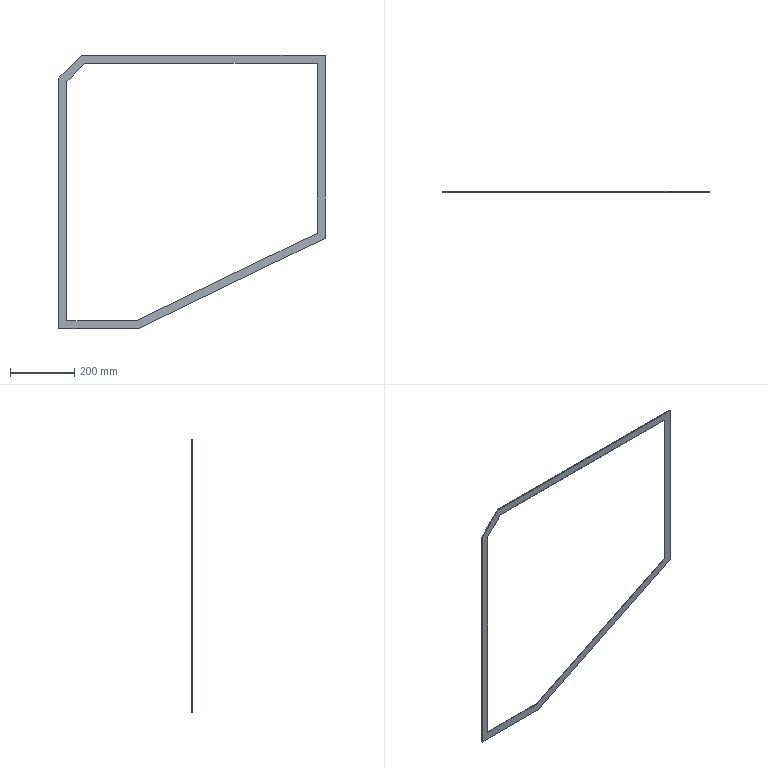Part | NX | features BREP 1 | 1 solid | 14 faces | box 830.914 x 2 x 852.689 mm | volume 150814 mm3 | plane 14
STEP:
#1=CARTESIAN_POINT('',(802.673,-691.5,466.003));
#2=VERTEX_POINT('',#1);
#3=CARTESIAN_POINT('',(802.673,-691.5,1212.752));
#4=VERTEX_POINT('',#3);
#5=CARTESIAN_POINT('',(802.673,-691.5,839.378));
#6=DIRECTION('',(0.,0.,1.));
#7=VECTOR('',#6,1000.);
#8=LINE('',#5,#7);
#9=EDGE_CURVE('',#2,#4,#8,.T.);
#10=ORIENTED_EDGE('',*,*,#9,.F.);
#11=CARTESIAN_POINT('',(802.673,-689.5,466.003));
#12=VERTEX_POINT('',#11);
#13=CARTESIAN_POINT('',(802.673,-690.5,466.003));
#14=DIRECTION('',(0.,-1.,0.));
#15=VECTOR('',#14,1000.);
#16=LINE('',#13,#15);
#17=EDGE_CURVE('',#12,#2,#16,.T.);
#18=ORIENTED_EDGE('',*,*,#17,.F.);
#19=CARTESIAN_POINT('',(802.673,-689.5,1212.752));
#20=VERTEX_POINT('',#19);
#21=CARTESIAN_POINT('',(802.673,-689.5,839.378));
#22=DIRECTION('',(0.,0.,1.));
#23=VECTOR('',#22,1000.);
#24=LINE('',#21,#23);
#25=EDGE_CURVE('',#12,#20,#24,.T.);
#26=ORIENTED_EDGE('',*,*,#25,.T.);
#27=CARTESIAN_POINT('',(802.673,-690.5,1212.752));
#28=DIRECTION('',(0.,-1.,0.));
#29=VECTOR('',#28,1000.);
#30=LINE('',#27,#29);
#31=EDGE_CURVE('',#20,#4,#30,.T.);
#32=ORIENTED_EDGE('',*,*,#31,.T.);
#33=EDGE_LOOP('',(#10,#18,#26,#32));
#34=FACE_BOUND('',#33,.T.);
#35=CARTESIAN_POINT('',(802.673,-691.5,839.378));
#36=DIRECTION('',(1.,0.,0.));
#37=DIRECTION('',(0.,0.,-1.));
#38=AXIS2_PLACEMENT_3D('',#35,#36,#37);
#39=PLANE('',#38);
#40=ADVANCED_FACE('',(#34),#39,.T.);
#41=CARTESIAN_POINT('',(1020.296,-691.5,466.003));
#42=VERTEX_POINT('',#41);
#43=CARTESIAN_POINT('',(911.485,-691.5,466.003));
#44=DIRECTION('',(1.,0.,0.));
#45=VECTOR('',#44,1000.);
#46=LINE('',#43,#45);
#47=EDGE_CURVE('',#2,#42,#46,.T.);
#48=ORIENTED_EDGE('',*,*,#47,.T.);
#49=CARTESIAN_POINT('',(1020.296,-689.5,466.003));
#50=VERTEX_POINT('',#49);
#51=CARTESIAN_POINT('',(1020.296,-690.5,466.003));
#52=DIRECTION('',(0.,1.,0.));
#53=VECTOR('',#52,1000.);
#54=LINE('',#51,#53);
#55=EDGE_CURVE('',#42,#50,#54,.T.);
#56=ORIENTED_EDGE('',*,*,#55,.T.);
#57=CARTESIAN_POINT('',(911.485,-689.5,466.003));
#58=DIRECTION('',(1.,0.,0.));
#59=VECTOR('',#58,1000.);
#60=LINE('',#57,#59);
#61=EDGE_CURVE('',#12,#50,#60,.T.);
#62=ORIENTED_EDGE('',*,*,#61,.F.);
#63=ORIENTED_EDGE('',*,*,#17,.T.);
#64=EDGE_LOOP('',(#48,#56,#62,#63));
#65=FACE_BOUND('',#64,.T.);
#66=CARTESIAN_POINT('',(911.485,-691.5,466.003));
#67=DIRECTION('',(0.,0.,1.));
#68=DIRECTION('',(1.,0.,0.));
#69=AXIS2_PLACEMENT_3D('',#66,#67,#68);
#70=PLANE('',#69);
#71=ADVANCED_FACE('',(#65),#70,.T.);
#72=CARTESIAN_POINT('',(1583.587,-691.5,738.903));
#73=VERTEX_POINT('',#72);
#74=CARTESIAN_POINT('',(1583.587,-689.5,738.903));
#75=VERTEX_POINT('',#74);
#76=CARTESIAN_POINT('',(1583.587,-690.5,738.903));
#77=DIRECTION('',(0.,1.,0.));
#78=VECTOR('',#77,1000.);
#79=LINE('',#76,#78);
#80=EDGE_CURVE('',#73,#75,#79,.T.);
#81=ORIENTED_EDGE('',*,*,#80,.T.);
#82=CARTESIAN_POINT('',(1301.942,-689.5,602.453));
#83=DIRECTION('',(0.8999,0.,0.436));
#84=VECTOR('',#83,1000.);
#85=LINE('',#82,#84);
#86=EDGE_CURVE('',#50,#75,#85,.T.);
#87=ORIENTED_EDGE('',*,*,#86,.F.);
#88=ORIENTED_EDGE('',*,*,#55,.F.);
#89=CARTESIAN_POINT('',(1301.942,-691.5,602.453));
#90=DIRECTION('',(0.8999,0.,0.436));
#91=VECTOR('',#90,1000.);
#92=LINE('',#89,#91);
#93=EDGE_CURVE('',#42,#73,#92,.T.);
#94=ORIENTED_EDGE('',*,*,#93,.T.);
#95=EDGE_LOOP('',(#81,#87,#88,#94));
#96=FACE_BOUND('',#95,.T.);
#97=CARTESIAN_POINT('',(1301.942,-691.5,602.453));
#98=DIRECTION('',(-0.436,0.,0.8999));
#99=DIRECTION('',(0.8999,0.,0.436));
#100=AXIS2_PLACEMENT_3D('',#97,#98,#99);
#101=PLANE('',#100);
#102=ADVANCED_FACE('',(#96),#101,.T.);
#103=CARTESIAN_POINT('',(1026.033,-691.5,441.003));
#104=VERTEX_POINT('',#103);
#105=CARTESIAN_POINT('',(1608.587,-691.5,723.235));
#106=VERTEX_POINT('',#105);
#107=CARTESIAN_POINT('',(1317.31,-691.5,582.119));
#108=DIRECTION('',(0.8999,0.,0.436));
#109=VECTOR('',#108,1000.);
#110=LINE('',#107,#109);
#111=EDGE_CURVE('',#104,#106,#110,.T.);
#112=ORIENTED_EDGE('',*,*,#111,.F.);
#113=CARTESIAN_POINT('',(1026.033,-689.5,441.003));
#114=VERTEX_POINT('',#113);
#115=CARTESIAN_POINT('',(1026.033,-690.5,441.003));
#116=DIRECTION('',(0.,1.,0.));
#117=VECTOR('',#116,1000.);
#118=LINE('',#115,#117);
#119=EDGE_CURVE('',#104,#114,#118,.T.);
#120=ORIENTED_EDGE('',*,*,#119,.T.);
#121=CARTESIAN_POINT('',(1608.587,-689.5,723.235));
#122=VERTEX_POINT('',#121);
#123=CARTESIAN_POINT('',(1317.31,-689.5,582.119));
#124=DIRECTION('',(0.8999,0.,0.436));
#125=VECTOR('',#124,1000.);
#126=LINE('',#123,#125);
#127=EDGE_CURVE('',#114,#122,#126,.T.);
#128=ORIENTED_EDGE('',*,*,#127,.T.);
#129=CARTESIAN_POINT('',(1608.587,-690.5,723.235));
#130=DIRECTION('',(0.,1.,0.));
#131=VECTOR('',#130,1000.);
#132=LINE('',#129,#131);
#133=EDGE_CURVE('',#106,#122,#132,.T.);
#134=ORIENTED_EDGE('',*,*,#133,.F.);
#135=EDGE_LOOP('',(#112,#120,#128,#134));
#136=FACE_BOUND('',#135,.T.);
#137=CARTESIAN_POINT('',(1317.31,-691.5,582.119));
#138=DIRECTION('',(-0.436,0.,0.8999));
#139=DIRECTION('',(0.8999,0.,0.436));
#140=AXIS2_PLACEMENT_3D('',#137,#138,#139);
#141=PLANE('',#140);
#142=ADVANCED_FACE('',(#136),#141,.F.);
#143=CARTESIAN_POINT('',(777.673,-691.5,441.003));
#144=VERTEX_POINT('',#143);
#145=CARTESIAN_POINT('',(901.853,-691.5,441.003));
#146=DIRECTION('',(1.,0.,0.));
#147=VECTOR('',#146,1000.);
#148=LINE('',#145,#147);
#149=EDGE_CURVE('',#144,#104,#148,.T.);
#150=ORIENTED_EDGE('',*,*,#149,.F.);
#151=CARTESIAN_POINT('',(777.673,-689.5,441.003));
#152=VERTEX_POINT('',#151);
#153=CARTESIAN_POINT('',(777.673,-691.5,441.003));
#154=DIRECTION('',(0.,-1.,0.));
#155=VECTOR('',#154,1000.);
#156=LINE('',#153,#155);
#157=EDGE_CURVE('',#152,#144,#156,.T.);
#158=ORIENTED_EDGE('',*,*,#157,.F.);
#159=CARTESIAN_POINT('',(901.853,-689.5,441.003));
#160=DIRECTION('',(1.,0.,0.));
#161=VECTOR('',#160,1000.);
#162=LINE('',#159,#161);
#163=EDGE_CURVE('',#152,#114,#162,.T.);
#164=ORIENTED_EDGE('',*,*,#163,.T.);
#165=ORIENTED_EDGE('',*,*,#119,.F.);
#166=EDGE_LOOP('',(#150,#158,#164,#165));
#167=FACE_BOUND('',#166,.T.);
#168=CARTESIAN_POINT('',(901.853,-691.5,441.003));
#169=DIRECTION('',(0.,0.,1.));
#170=DIRECTION('',(1.,0.,0.));
#171=AXIS2_PLACEMENT_3D('',#168,#169,#170);
#172=PLANE('',#171);
#173=ADVANCED_FACE('',(#167),#172,.F.);
#174=CARTESIAN_POINT('',(777.673,-689.5,1223.108));
#175=VERTEX_POINT('',#174);
#176=CARTESIAN_POINT('',(777.673,-691.5,1223.108));
#177=VERTEX_POINT('',#176);
#178=CARTESIAN_POINT('',(777.673,-690.5,1223.108));
#179=DIRECTION('',(0.,-1.,0.));
#180=VECTOR('',#179,1000.);
#181=LINE('',#178,#180);
#182=EDGE_CURVE('',#175,#177,#181,.T.);
#183=ORIENTED_EDGE('',*,*,#182,.F.);
#184=CARTESIAN_POINT('',(777.673,-689.5,832.055));
#185=DIRECTION('',(0.,0.,1.));
#186=VECTOR('',#185,1000.);
#187=LINE('',#184,#186);
#188=EDGE_CURVE('',#152,#175,#187,.T.);
#189=ORIENTED_EDGE('',*,*,#188,.F.);
#190=ORIENTED_EDGE('',*,*,#157,.T.);
#191=CARTESIAN_POINT('',(777.673,-691.5,832.055));
#192=DIRECTION('',(0.,0.,1.));
#193=VECTOR('',#192,1000.);
#194=LINE('',#191,#193);
#195=EDGE_CURVE('',#144,#177,#194,.T.);
#196=ORIENTED_EDGE('',*,*,#195,.T.);
#197=EDGE_LOOP('',(#183,#189,#190,#196));
#198=FACE_BOUND('',#197,.T.);
#199=CARTESIAN_POINT('',(777.673,-691.5,832.055));
#200=DIRECTION('',(1.,0.,0.));
#201=DIRECTION('',(0.,0.,-1.));
#202=AXIS2_PLACEMENT_3D('',#199,#200,#201);
#203=PLANE('',#202);
#204=ADVANCED_FACE('',(#198),#203,.F.);
#205=CARTESIAN_POINT('',(848.258,-691.5,1293.692));
#206=VERTEX_POINT('',#205);
#207=CARTESIAN_POINT('',(848.258,-689.5,1293.692));
#208=VERTEX_POINT('',#207);
#209=CARTESIAN_POINT('',(848.258,-690.5,1293.692));
#210=DIRECTION('',(0.,1.,0.));
#211=VECTOR('',#210,1000.);
#212=LINE('',#209,#211);
#213=EDGE_CURVE('',#206,#208,#212,.T.);
#214=ORIENTED_EDGE('',*,*,#213,.T.);
#215=CARTESIAN_POINT('',(812.966,-689.5,1258.4));
#216=DIRECTION('',(0.7071,0.,0.7071));
#217=VECTOR('',#216,1000.);
#218=LINE('',#215,#217);
#219=EDGE_CURVE('',#175,#208,#218,.T.);
#220=ORIENTED_EDGE('',*,*,#219,.F.);
#221=ORIENTED_EDGE('',*,*,#182,.T.);
#222=CARTESIAN_POINT('',(812.966,-691.5,1258.4));
#223=DIRECTION('',(0.7071,0.,0.7071));
#224=VECTOR('',#223,1000.);
#225=LINE('',#222,#224);
#226=EDGE_CURVE('',#177,#206,#225,.T.);
#227=ORIENTED_EDGE('',*,*,#226,.T.);
#228=EDGE_LOOP('',(#214,#220,#221,#227));
#229=FACE_BOUND('',#228,.T.);
#230=CARTESIAN_POINT('',(812.966,-691.5,1258.4));
#231=DIRECTION('',(-0.7071,0.,0.7071));
#232=DIRECTION('',(0.7071,0.,0.7071));
#233=AXIS2_PLACEMENT_3D('',#230,#231,#232);
#234=PLANE('',#233);
#235=ADVANCED_FACE('',(#229),#234,.T.);
#236=CARTESIAN_POINT('',(1608.587,-691.5,1293.692));
#237=VERTEX_POINT('',#236);
#238=CARTESIAN_POINT('',(1228.423,-691.5,1293.692));
#239=DIRECTION('',(1.,0.,0.));
#240=VECTOR('',#239,1000.);
#241=LINE('',#238,#240);
#242=EDGE_CURVE('',#206,#237,#241,.T.);
#243=ORIENTED_EDGE('',*,*,#242,.T.);
#244=CARTESIAN_POINT('',(1608.587,-689.5,1293.692));
#245=VERTEX_POINT('',#244);
#246=CARTESIAN_POINT('',(1608.587,-690.5,1293.692));
#247=DIRECTION('',(0.,1.,0.));
#248=VECTOR('',#247,1000.);
#249=LINE('',#246,#248);
#250=EDGE_CURVE('',#237,#245,#249,.T.);
#251=ORIENTED_EDGE('',*,*,#250,.T.);
#252=CARTESIAN_POINT('',(1228.423,-689.5,1293.692));
#253=DIRECTION('',(1.,0.,0.));
#254=VECTOR('',#253,1000.);
#255=LINE('',#252,#254);
#256=EDGE_CURVE('',#208,#245,#255,.T.);
#257=ORIENTED_EDGE('',*,*,#256,.F.);
#258=ORIENTED_EDGE('',*,*,#213,.F.);
#259=EDGE_LOOP('',(#243,#251,#257,#258));
#260=FACE_BOUND('',#259,.T.);
#261=CARTESIAN_POINT('',(1228.423,-691.5,1293.692));
#262=DIRECTION('',(0.,0.,1.));
#263=DIRECTION('',(1.,0.,0.));
#264=AXIS2_PLACEMENT_3D('',#261,#262,#263);
#265=PLANE('',#264);
#266=ADVANCED_FACE('',(#260),#265,.T.);
#267=CARTESIAN_POINT('',(1608.587,-691.5,1008.463));
#268=DIRECTION('',(0.,0.,-1.));
#269=VECTOR('',#268,1000.);
#270=LINE('',#267,#269);
#271=EDGE_CURVE('',#237,#106,#270,.T.);
#272=ORIENTED_EDGE('',*,*,#271,.T.);
#273=ORIENTED_EDGE('',*,*,#133,.T.);
#274=CARTESIAN_POINT('',(1608.587,-689.5,1008.463));
#275=DIRECTION('',(0.,0.,-1.));
#276=VECTOR('',#275,1000.);
#277=LINE('',#274,#276);
#278=EDGE_CURVE('',#245,#122,#277,.T.);
#279=ORIENTED_EDGE('',*,*,#278,.F.);
#280=ORIENTED_EDGE('',*,*,#250,.F.);
#281=EDGE_LOOP('',(#272,#273,#279,#280));
#282=FACE_BOUND('',#281,.T.);
#283=CARTESIAN_POINT('',(1608.587,-691.5,1008.463));
#284=DIRECTION('',(-1.,0.,0.));
#285=DIRECTION('',(0.,1.,0.));
#286=AXIS2_PLACEMENT_3D('',#283,#284,#285);
#287=PLANE('',#286);
#288=ADVANCED_FACE('',(#282),#287,.F.);
#289=CARTESIAN_POINT('',(1583.587,-691.5,1268.692));
#290=VERTEX_POINT('',#289);
#291=CARTESIAN_POINT('',(1583.587,-689.5,1268.692));
#292=VERTEX_POINT('',#291);
#293=CARTESIAN_POINT('',(1583.587,-690.5,1268.692));
#294=DIRECTION('',(0.,1.,0.));
#295=VECTOR('',#294,1000.);
#296=LINE('',#293,#295);
#297=EDGE_CURVE('',#290,#292,#296,.T.);
#298=ORIENTED_EDGE('',*,*,#297,.T.);
#299=CARTESIAN_POINT('',(1583.587,-689.5,1003.797));
#300=DIRECTION('',(0.,0.,-1.));
#301=VECTOR('',#300,1000.);
#302=LINE('',#299,#301);
#303=EDGE_CURVE('',#292,#75,#302,.T.);
#304=ORIENTED_EDGE('',*,*,#303,.T.);
#305=ORIENTED_EDGE('',*,*,#80,.F.);
#306=CARTESIAN_POINT('',(1583.587,-691.5,1003.797));
#307=DIRECTION('',(0.,0.,-1.));
#308=VECTOR('',#307,1000.);
#309=LINE('',#306,#308);
#310=EDGE_CURVE('',#290,#73,#309,.T.);
#311=ORIENTED_EDGE('',*,*,#310,.F.);
#312=EDGE_LOOP('',(#298,#304,#305,#311));
#313=FACE_BOUND('',#312,.T.);
#314=CARTESIAN_POINT('',(1583.587,-691.5,1003.797));
#315=DIRECTION('',(-1.,0.,0.));
#316=DIRECTION('',(0.,1.,0.));
#317=AXIS2_PLACEMENT_3D('',#314,#315,#316);
#318=PLANE('',#317);
#319=ADVANCED_FACE('',(#313),#318,.T.);
#320=ORIENTED_EDGE('',*,*,#25,.F.);
#321=ORIENTED_EDGE('',*,*,#61,.T.);
#322=ORIENTED_EDGE('',*,*,#86,.T.);
#323=ORIENTED_EDGE('',*,*,#303,.F.);
#324=CARTESIAN_POINT('',(858.613,-689.5,1268.692));
#325=VERTEX_POINT('',#324);
#326=CARTESIAN_POINT('',(1221.1,-689.5,1268.692));
#327=DIRECTION('',(1.,0.,0.));
#328=VECTOR('',#327,1000.);
#329=LINE('',#326,#328);
#330=EDGE_CURVE('',#325,#292,#329,.T.);
#331=ORIENTED_EDGE('',*,*,#330,.F.);
#332=CARTESIAN_POINT('',(830.643,-689.5,1240.722));
#333=DIRECTION('',(0.7071,0.,0.7071));
#334=VECTOR('',#333,1000.);
#335=LINE('',#332,#334);
#336=EDGE_CURVE('',#20,#325,#335,.T.);
#337=ORIENTED_EDGE('',*,*,#336,.F.);
#338=EDGE_LOOP('',(#320,#321,#322,#323,#331,#337));
#339=FACE_BOUND('',#338,.T.);
#340=ORIENTED_EDGE('',*,*,#127,.F.);
#341=ORIENTED_EDGE('',*,*,#163,.F.);
#342=ORIENTED_EDGE('',*,*,#188,.T.);
#343=ORIENTED_EDGE('',*,*,#219,.T.);
#344=ORIENTED_EDGE('',*,*,#256,.T.);
#345=ORIENTED_EDGE('',*,*,#278,.T.);
#346=EDGE_LOOP('',(#340,#341,#342,#343,#344,#345));
#347=FACE_BOUND('',#346,.T.);
#348=CARTESIAN_POINT('',(1116.267,-689.5,781.39));
#349=DIRECTION('',(0.,-1.,0.));
#350=DIRECTION('',(-0.1176,0.,0.9931));
#351=AXIS2_PLACEMENT_3D('',#348,#349,#350);
#352=PLANE('',#351);
#353=ADVANCED_FACE('',(#339,#347),#352,.F.);
#354=CARTESIAN_POINT('',(858.613,-691.5,1268.692));
#355=VERTEX_POINT('',#354);
#356=CARTESIAN_POINT('',(830.643,-691.5,1240.722));
#357=DIRECTION('',(0.7071,0.,0.7071));
#358=VECTOR('',#357,1000.);
#359=LINE('',#356,#358);
#360=EDGE_CURVE('',#4,#355,#359,.T.);
#361=ORIENTED_EDGE('',*,*,#360,.F.);
#362=ORIENTED_EDGE('',*,*,#31,.F.);
#363=ORIENTED_EDGE('',*,*,#336,.T.);
#364=CARTESIAN_POINT('',(858.613,-690.5,1268.692));
#365=DIRECTION('',(0.,1.,0.));
#366=VECTOR('',#365,1000.);
#367=LINE('',#364,#366);
#368=EDGE_CURVE('',#355,#325,#367,.T.);
#369=ORIENTED_EDGE('',*,*,#368,.F.);
#370=EDGE_LOOP('',(#361,#362,#363,#369));
#371=FACE_BOUND('',#370,.T.);
#372=CARTESIAN_POINT('',(830.643,-691.5,1240.722));
#373=DIRECTION('',(-0.7071,0.,0.7071));
#374=DIRECTION('',(0.7071,0.,0.7071));
#375=AXIS2_PLACEMENT_3D('',#372,#373,#374);
#376=PLANE('',#375);
#377=ADVANCED_FACE('',(#371),#376,.F.);
#378=ORIENTED_EDGE('',*,*,#360,.T.);
#379=CARTESIAN_POINT('',(1221.1,-691.5,1268.692));
#380=DIRECTION('',(1.,0.,0.));
#381=VECTOR('',#380,1000.);
#382=LINE('',#379,#381);
#383=EDGE_CURVE('',#355,#290,#382,.T.);
#384=ORIENTED_EDGE('',*,*,#383,.T.);
#385=ORIENTED_EDGE('',*,*,#310,.T.);
#386=ORIENTED_EDGE('',*,*,#93,.F.);
#387=ORIENTED_EDGE('',*,*,#47,.F.);
#388=ORIENTED_EDGE('',*,*,#9,.T.);
#389=EDGE_LOOP('',(#378,#384,#385,#386,#387,#388));
#390=FACE_BOUND('',#389,.T.);
#391=ORIENTED_EDGE('',*,*,#271,.F.);
#392=ORIENTED_EDGE('',*,*,#242,.F.);
#393=ORIENTED_EDGE('',*,*,#226,.F.);
#394=ORIENTED_EDGE('',*,*,#195,.F.);
#395=ORIENTED_EDGE('',*,*,#149,.T.);
#396=ORIENTED_EDGE('',*,*,#111,.T.);
#397=EDGE_LOOP('',(#391,#392,#393,#394,#395,#396));
#398=FACE_BOUND('',#397,.T.);
#399=CARTESIAN_POINT('',(1116.267,-691.5,781.39));
#400=DIRECTION('',(0.,-1.,0.));
#401=DIRECTION('',(-0.1176,0.,0.9931));
#402=AXIS2_PLACEMENT_3D('',#399,#400,#401);
#403=PLANE('',#402);
#404=ADVANCED_FACE('',(#390,#398),#403,.T.);
#405=ORIENTED_EDGE('',*,*,#383,.F.);
#406=ORIENTED_EDGE('',*,*,#368,.T.);
#407=ORIENTED_EDGE('',*,*,#330,.T.);
#408=ORIENTED_EDGE('',*,*,#297,.F.);
#409=EDGE_LOOP('',(#405,#406,#407,#408));
#410=FACE_BOUND('',#409,.T.);
#411=CARTESIAN_POINT('',(1221.1,-691.5,1268.692));
#412=DIRECTION('',(0.,0.,1.));
#413=DIRECTION('',(1.,0.,0.));
#414=AXIS2_PLACEMENT_3D('',#411,#412,#413);
#415=PLANE('',#414);
#416=ADVANCED_FACE('',(#410),#415,.F.);
#417=CLOSED_SHELL('',(#40,#71,#102,#142,#173,#204,#235,#266,#288,#319,#353,#377,#404,#416));
#418=MANIFOLD_SOLID_BREP('',#417);
#419=(LENGTH_UNIT()NAMED_UNIT(*)SI_UNIT(.MILLI.,.METRE.));
#420=UNCERTAINTY_MEASURE_WITH_UNIT(LENGTH_MEASURE(0.00001),#419,'','');
#421=(NAMED_UNIT(*)PLANE_ANGLE_UNIT()SI_UNIT($,.RADIAN.));
#422=(NAMED_UNIT(*)SI_UNIT($,.STERADIAN.)SOLID_ANGLE_UNIT());
#423=(GEOMETRIC_REPRESENTATION_CONTEXT(3)GLOBAL_UNCERTAINTY_ASSIGNED_CONTEXT((#420))GLOBAL_UNIT_ASSIGNED_CONTEXT((#419,#421,#422))REPRESENTATION_CONTEXT('',''));
#424=ADVANCED_BREP_SHAPE_REPRESENTATION('',(#418),#423);